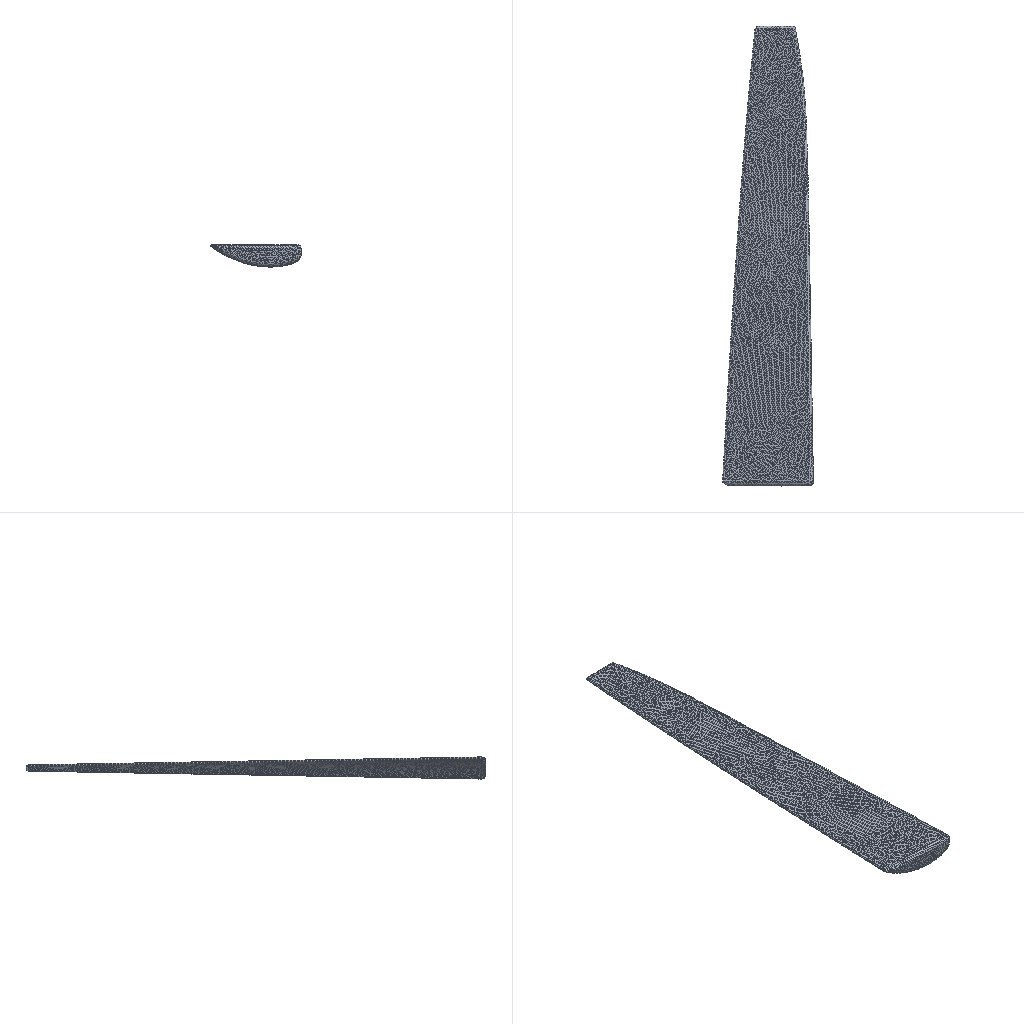Simulation study | ansys workbench
Set-up summary:
category,name,step,type,value,unit,region
solver,ansys_workbench
units,mm-N-s-tonne (MPa),,stated,"/units,MPA"
analysis,LS1,,static
load_step,LS1,LS1,static,nsubst=1; time=1
mesh,nodes,,,110262
mesh,elements,,,85509
element_type,SOLID187,,,62516
element_type,SURF154,,,22993
material,Structural Steel,,E,200000,tonne s^-2 mm^-1
material,Structural Steel,,nu,0.3
material,Structural Steel,,density,7.85e-09,tonne mm^-3
material,Structural Steel,,conductivity,60.5,tonne mm s^-3 C^-1
material,Structural Steel,,specific_heat,4.34e+08,mm^2 s^-2 C^-1
material,Structural Steel,,cte,1.2e-05,C^-1
material,Structural Steel,,permeability,10000
material,Structural Steel,,resistivity,0.00017,ohm mm
load,Define Force Using Surface Effect Elements,LS1,surface-effect pres face 1,0.0006836,,SURF154 #2
load,Define Force Using Surface Effect Elements,LS1,surface-effect pres face 3,-5.31531e-20,,SURF154 #2
bc,Fixed Supports,model,fixed,[dofs=ALL],,_FIXEDSU
named_set,_FIXEDSU,,node,684
Ansys APDL input file, long lists of numbers shortened:
/batch
/config,noeldb,1     ! force off writing results to database
*get,_wallstrt,active,,time,wall
! ANSYS input file written by Workbench version 2022 R1
! File used for geometry attach:
/title,wbnew--____ (B5)
! ****** Begin Custom Load Command Snippet ******
/COM, ACT Extensions:
/COM,     LSDYNA, 2021.1
/COM,
! ****** End   Custom Load Command Snippet ******
*DIM,_wb_ProjectScratch_dir,string,248
_wb_ProjectScratch_dir(1) = ''
*DIM,_wb_SolverFiles_dir,string,248
_wb_SolverFiles_dir(1) = ''
*DIM,_wb_userfiles_dir,string,248
_wb_userfiles_dir(1) = ''
/com,--- Data in consistent NMM units. See Solving Units in the help system for more information.
/units,MPA
/nopr
/wb,file,start              !  signify a WB generated input file
/prep7
! Turn off shape checking because checks already performed inside WB mesher.
! See help system for more information.
SHPP,OFF,,NOWARN
/nolist
etcon,set             ! allow ANSYS to choose best KEYOP's for 180x elements, resets any applicable keyopt to MAPDL defaults
/com,*********** Nodes for the whole assembly ***********
nblock,3,,121288
(1i9,3e20.9e3)
        1     9.596826886E+03     0.000000000E+00    -5.088036965E+02
! (110261 more lines like these left out)
-1
/wb,elem,start            !  set before creation of elements
/com,*********** Elements for Body 1 "__1-FreeParts|__6" ***********
et,1,187
eblock,19,solid,,62516
(19i9)
        1        1        1        1        0        0        0        0       10        0        1     3895    15310    17455    17344    45565   105324    45569    45567
! (125031 more lines like these left out)
-1
/wb,elem,end               !  done creating elements
/com,*********** Send User Defined Coordinate System(s) ***********
csys,0
toffst,273.15,  ! Temperature offset from absolute zero
/com,*********** Set Reference Temperature ***********
tref,22.
/wb,mat,start              !  starting to send materials
/com,*********** Send Materials ***********
Temperature = 'TEMP' ! Temperature
MP,DENS,1,7.85e-09,	! tonne mm^-3
MP,ALPX,1,1.2e-05,	! C^-1
MP,C,1,434000000,	! mm^2 s^-2 C^-1
MP,KXX,1,60.5,	! tonne mm s^-3 C^-1
MP,RSVX,1,0.00017,	! ohm mm
MP,EX,1,200000,	! tonne s^-2 mm^-1
MP,NUXY,1,0.3,
MP,MURX,1,10000,
/wb,mat,end                !  done sending materials
!************************* Model Summary ********************
!__1-FreeParts|__6,	结构钢,	matid,	1
!************************* End Model Summary ********************
! get the diagonal of the bounding box. Needed later for other things
*get,_xmin,node,,mnloc,x
*get,_ymin,node,,mnloc,y
*get,_zmin,node,,mnloc,z
*get,_xmax,node,,mxloc,x
*get,_ymax,node,,mxloc,y
*get,_zmax,node,,mxloc,z
_ASMDIAG=(_xmax-_xmin)*(_xmax-_xmin)+(_ymax-_ymin)*(_ymax-_ymin)+(_zmax-_zmin)*(_zmax-_zmin)
_ASMDIAG=SQRT(_ASMDIAG)
/wb,contact,start          !  starting to send contact
/wb,contact,end            !  done creating contacts
/golist
/wb,load,start             !  starting to send loads
/com,*********** Fixed Supports ***********
CMBLOCK,_FIXEDSU,NODE,      684
(8i10)
         1         7        17        18        19        20        21        22
! (85 more lines like these left out)
cmsel,s,_FIXEDSU
d,all,all
nsel,all
/com,*********** Define Force Using Surface Effect Elements ***********
local,12,0,0.,0.,0.,0.,0.,0.
csys,0
et,2,154
eblock,10,,,22993
(15i9)
    88191        2        2        2       12     1420     1419     7822     7822    26387    26388     7822    26394
! (22992 more lines like these left out)
-1
esel,s,type,,2
keyop,2,2,1                ! Apply load in local coordinate system
keyop,2,7,1                ! Use original area so load is constant in large deformation
esel,all
/gst,on,on
fini
*get,_numnode,node,0,count
*get,_numelem,elem,0,count
*get, _MAXELEMNUM, elem, 0, NUM, MAX
*get, _MAXNODENUM, node, 0, NUM, MAX
*get, _MAXELEMTYPE, etyp, 0, NUM, MAX
*get, _MAXREALCONST, real, 0, NUM, MAX
/go
/wb,load,end               !  done creating loads
/com,--- Number of total nodes = %_numnode%
/com,--- Number of contact elements = 22993
/com,--- Number of spring elements = 0
/com,--- Number of bearing elements = 0
/com,--- Number of solid elements = 62516
/com,--- Number of condensed parts = 0
/com,--- Number of total elements = %_numelem%
*get,_wallbsol,active,,time,wall
/com,****************************************************************************
/com,*************************    SOLUTION       ********************************
/com,****************************************************************************
/solu
antype,0                   ! static analysis
_thickRatio=  1     ! Ratio of thick parts in the model
eqsl,pcg,1e-8,,,,,,1
cntr,print,1               ! print out contact info and also make no initial contact an error
dmpoption,emat,no             ! Don't combine emat file for DANSYS
dmpoption,esav,no             ! Don't combine esav file for DANSYS
nldiag,cont,iter           ! print out contact info each equilibrium iteration
rescontrol,,none                 ! Do not keep any restart files
/com,****************************************************
/com,******************* SOLVE FOR LS 1 OF 1 ****************
esel,s,type,,2
nsle
sfe,all,1,pres,1,6.83557683289664e-004
sfe,all,2,pres,1,0.
sfe,all,3,pres,1,-5.31530837310164e-020
nsel,all
esel,all
/nopr
/gopr
nsub,1,1,1
time,1.
outres,erase
outres,all,none
outres,nsol,all,
outres,rsol,all
outres,eangl,all
outres,etmp,all
outres,veng,all
outres,strs,all,
outres,epel,all,
outres,eppl,all,
outres,cont,all,
! *********** WB SOLVE COMMAND ***********
! check interactive state
*get,ANSINTER_,active,,int
*if,ANSINTER_,ne,0,then
/eof
*endif
solve
/com *************** Write FE CONNECTORS *********
CEWRITE,file,ce,,INTE
/com,****************************************************
/com,*************** FINISHED SOLVE FOR LS 1 *************
*get,_wallasol,active,,time,wall
/nopr
*get,_numnode,node,0,count
*get,_numelem,elem,0,count
*get, _MAXELEMNUM, elem, 0, NUM, MAX
*get, _MAXNODENUM, node, 0, NUM, MAX,,,INTERNAL
*get, _MAXELEMTYPE, etyp, 0, NUM, MAX
*get, _MAXREALCONST, real, 0, NUM, MAX
/gopr
*get,_PCGITER,active,,solu,cgiter
/post1
xmlo,ENCODING,ISO-8859-1
xmlo,parm
/xml,parm,xml
fini
/gopr
*get,_walldone,active,,time,wall
_preptime=(_wallbsol-_wallstrt)*3600
_solvtime=(_wallasol-_wallbsol)*3600
_posttime=(_walldone-_wallasol)*3600
_totaltim=(_walldone-_wallstrt)*3600
*get,_dlbratio,active,0,solu,dlbr
*get,_combtime,active,0,solu,comb
*get,_ssmode,active,0,solu,ssmm
*get,_ndofs,active,0,solu,ndof
*get,_sol_end_time,active,0,set,time
*if,_sol_end_time,eq,1.,then
/fclean				!clean distributed files
*endif
/com,--- Total number of nodes = %_numnode%
/com,--- Total number of elements = %_numelem%
/com,--- Element load balance ratio = %_dlbratio%
/com,--- Time to combine distributed files = %_combtime%
/com,--- Sparse memory mode = %_ssmode%
/com,--- Number of DOF = %_ndofs%
/wb,file,end               ! done with WB generated input
Results summary:
result,analyses[0].index,,,1
result,analyses[0].system,,,SYS
result,analyses[0].deck,,,deck.dat
result,analyses[0].solve_status,,,completed
result,analyses[0].analysis_type,,,static
result,analyses[0].physics,,,mechanical
result,analyses[0].unit_system,,,"NMM: mm, ton, N, s, mV, mA, degC"
result,analyses[0].n_sets,,,1
result,analyses[0].load_steps[0].set,set=1,,1
result,analyses[0].load_steps[0].time_or_freq,set=1,,1
result,analyses[0].load_steps[0].max_displacement_magnitude,set=1,,0.7481
result,analyses[0].load_steps[0].max_von_mises_nodal,set=1,,3.693
result,analyses[0].load_steps[0].reaction_force_sum_xyz[1],set=1,,-543471
result,analyses[0].load_steps[0].reaction_force_sum_xyz[2],set=1,,-0.001927
result,analyses[0].load_steps[0].reaction_force_sum_xyz[3],set=1,,0.002755